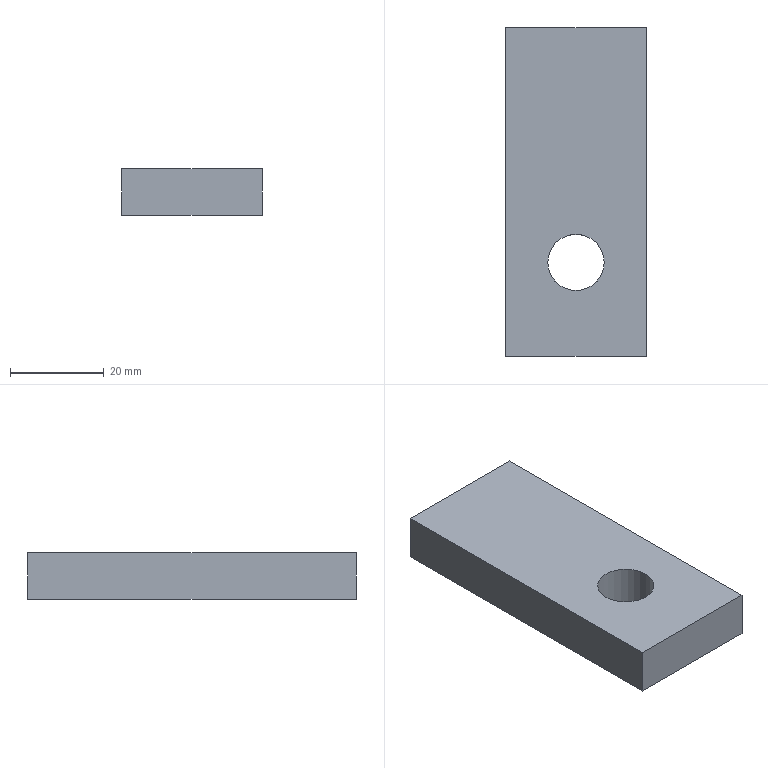Part | NX | features solid 2 | 1 solid | 7 faces | box 30 x 70 x 10 mm | volume 19869 mm3 | plane 6 | cylinder 1 | commonest cylinder face diameters 12 x1
STEP:
#1=CARTESIAN_POINT('',(664.,10.,-75.));
#2=VERTEX_POINT('',#1);
#3=CARTESIAN_POINT('',(670.,10.,-75.));
#4=DIRECTION('',(0.,0.,-1.));
#5=DIRECTION('',(-1.,0.,0.));
#6=AXIS2_PLACEMENT_3D('',#3,#4,#5);
#7=CIRCLE('',#6,6.);
#8=EDGE_CURVE('',#2,#2,#7,.F.);
#9=ORIENTED_EDGE('',*,*,#8,.F.);
#10=EDGE_LOOP('',(#9));
#11=FACE_BOUND('',#10,.T.);
#12=CARTESIAN_POINT('',(664.,10.,-65.));
#13=VERTEX_POINT('',#12);
#14=CARTESIAN_POINT('',(670.,10.,-65.));
#15=DIRECTION('',(0.,0.,-1.));
#16=DIRECTION('',(-1.,0.,0.));
#17=AXIS2_PLACEMENT_3D('',#14,#15,#16);
#18=CIRCLE('',#17,6.);
#19=EDGE_CURVE('',#13,#13,#18,.F.);
#20=ORIENTED_EDGE('',*,*,#19,.T.);
#21=EDGE_LOOP('',(#20));
#22=FACE_BOUND('',#21,.T.);
#23=CARTESIAN_POINT('',(670.,10.,-10.));
#24=DIRECTION('',(0.,0.,-1.));
#25=DIRECTION('',(-1.,0.,0.));
#26=AXIS2_PLACEMENT_3D('',#23,#24,#25);
#27=CYLINDRICAL_SURFACE('',#26,6.);
#28=ADVANCED_FACE('',(#11,#22),#27,.F.);
#29=CARTESIAN_POINT('',(685.,-10.,-65.));
#30=VERTEX_POINT('',#29);
#31=CARTESIAN_POINT('',(685.,-10.,-75.));
#32=VERTEX_POINT('',#31);
#33=CARTESIAN_POINT('',(685.,-10.,-10.));
#34=DIRECTION('',(0.,0.,1.));
#35=VECTOR('',#34,1000.);
#36=LINE('',#33,#35);
#37=EDGE_CURVE('',#30,#32,#36,.F.);
#38=ORIENTED_EDGE('',*,*,#37,.F.);
#39=CARTESIAN_POINT('',(655.,-10.,-65.));
#40=VERTEX_POINT('',#39);
#41=CARTESIAN_POINT('',(585.,-10.,-65.));
#42=DIRECTION('',(1.,0.,0.));
#43=VECTOR('',#42,1000.);
#44=LINE('',#41,#43);
#45=EDGE_CURVE('',#40,#30,#44,.T.);
#46=ORIENTED_EDGE('',*,*,#45,.F.);
#47=CARTESIAN_POINT('',(655.,-10.,-75.));
#48=VERTEX_POINT('',#47);
#49=CARTESIAN_POINT('',(655.,-10.,-10.));
#50=DIRECTION('',(0.,0.,1.));
#51=VECTOR('',#50,1000.);
#52=LINE('',#49,#51);
#53=EDGE_CURVE('',#40,#48,#52,.F.);
#54=ORIENTED_EDGE('',*,*,#53,.T.);
#55=CARTESIAN_POINT('',(585.,-10.,-75.));
#56=DIRECTION('',(1.,0.,0.));
#57=VECTOR('',#56,1000.);
#58=LINE('',#55,#57);
#59=EDGE_CURVE('',#32,#48,#58,.F.);
#60=ORIENTED_EDGE('',*,*,#59,.F.);
#61=EDGE_LOOP('',(#38,#46,#54,#60));
#62=FACE_BOUND('',#61,.T.);
#63=CARTESIAN_POINT('',(685.,-10.,-10.));
#64=DIRECTION('',(0.,1.,0.));
#65=DIRECTION('',(0.,0.,1.));
#66=AXIS2_PLACEMENT_3D('',#63,#64,#65);
#67=PLANE('',#66);
#68=ADVANCED_FACE('',(#62),#67,.F.);
#69=ORIENTED_EDGE('',*,*,#53,.F.);
#70=CARTESIAN_POINT('',(655.,60.,-65.));
#71=VERTEX_POINT('',#70);
#72=CARTESIAN_POINT('',(655.,90.,-65.));
#73=DIRECTION('',(0.,1.,0.));
#74=VECTOR('',#73,1000.);
#75=LINE('',#72,#74);
#76=EDGE_CURVE('',#71,#40,#75,.F.);
#77=ORIENTED_EDGE('',*,*,#76,.F.);
#78=CARTESIAN_POINT('',(655.,60.,-75.));
#79=VERTEX_POINT('',#78);
#80=CARTESIAN_POINT('',(655.,60.,-10.));
#81=DIRECTION('',(0.,0.,1.));
#82=VECTOR('',#81,1000.);
#83=LINE('',#80,#82);
#84=EDGE_CURVE('',#71,#79,#83,.F.);
#85=ORIENTED_EDGE('',*,*,#84,.T.);
#86=CARTESIAN_POINT('',(655.,205.,-75.));
#87=DIRECTION('',(0.,1.,0.));
#88=VECTOR('',#87,1000.);
#89=LINE('',#86,#88);
#90=EDGE_CURVE('',#79,#48,#89,.F.);
#91=ORIENTED_EDGE('',*,*,#90,.T.);
#92=EDGE_LOOP('',(#69,#77,#85,#91));
#93=FACE_BOUND('',#92,.T.);
#94=CARTESIAN_POINT('',(655.,205.,-10.));
#95=DIRECTION('',(1.,0.,0.));
#96=DIRECTION('',(0.,0.,-1.));
#97=AXIS2_PLACEMENT_3D('',#94,#95,#96);
#98=PLANE('',#97);
#99=ADVANCED_FACE('',(#93),#98,.F.);
#100=CARTESIAN_POINT('',(685.,60.,-75.));
#101=VERTEX_POINT('',#100);
#102=CARTESIAN_POINT('',(685.,205.,-75.));
#103=DIRECTION('',(0.,1.,0.));
#104=VECTOR('',#103,1000.);
#105=LINE('',#102,#104);
#106=EDGE_CURVE('',#101,#32,#105,.F.);
#107=ORIENTED_EDGE('',*,*,#106,.F.);
#108=CARTESIAN_POINT('',(685.,60.,-65.));
#109=VERTEX_POINT('',#108);
#110=CARTESIAN_POINT('',(685.,60.,-10.));
#111=DIRECTION('',(0.,0.,-1.));
#112=VECTOR('',#111,1000.);
#113=LINE('',#110,#112);
#114=EDGE_CURVE('',#101,#109,#113,.F.);
#115=ORIENTED_EDGE('',*,*,#114,.T.);
#116=CARTESIAN_POINT('',(685.,90.,-65.));
#117=DIRECTION('',(0.,1.,0.));
#118=VECTOR('',#117,1000.);
#119=LINE('',#116,#118);
#120=EDGE_CURVE('',#109,#30,#119,.F.);
#121=ORIENTED_EDGE('',*,*,#120,.T.);
#122=ORIENTED_EDGE('',*,*,#37,.T.);
#123=EDGE_LOOP('',(#107,#115,#121,#122));
#124=FACE_BOUND('',#123,.T.);
#125=CARTESIAN_POINT('',(685.,205.,-10.));
#126=DIRECTION('',(1.,0.,0.));
#127=DIRECTION('',(0.,0.,-1.));
#128=AXIS2_PLACEMENT_3D('',#125,#126,#127);
#129=PLANE('',#128);
#130=ADVANCED_FACE('',(#124),#129,.T.);
#131=ORIENTED_EDGE('',*,*,#120,.F.);
#132=CARTESIAN_POINT('',(585.,60.,-65.));
#133=DIRECTION('',(-1.,0.,0.));
#134=VECTOR('',#133,1000.);
#135=LINE('',#132,#134);
#136=EDGE_CURVE('',#109,#71,#135,.T.);
#137=ORIENTED_EDGE('',*,*,#136,.T.);
#138=ORIENTED_EDGE('',*,*,#76,.T.);
#139=ORIENTED_EDGE('',*,*,#45,.T.);
#140=EDGE_LOOP('',(#131,#137,#138,#139));
#141=FACE_BOUND('',#140,.T.);
#142=ORIENTED_EDGE('',*,*,#19,.F.);
#143=EDGE_LOOP('',(#142));
#144=FACE_BOUND('',#143,.T.);
#145=CARTESIAN_POINT('',(585.,225.,-65.));
#146=DIRECTION('',(0.,0.,-1.));
#147=DIRECTION('',(0.,1.,0.));
#148=AXIS2_PLACEMENT_3D('',#145,#146,#147);
#149=PLANE('',#148);
#150=ADVANCED_FACE('',(#141,#144),#149,.F.);
#151=ORIENTED_EDGE('',*,*,#90,.F.);
#152=CARTESIAN_POINT('',(585.,60.,-75.));
#153=DIRECTION('',(-1.,0.,0.));
#154=VECTOR('',#153,1000.);
#155=LINE('',#152,#154);
#156=EDGE_CURVE('',#79,#101,#155,.F.);
#157=ORIENTED_EDGE('',*,*,#156,.T.);
#158=ORIENTED_EDGE('',*,*,#106,.T.);
#159=ORIENTED_EDGE('',*,*,#59,.T.);
#160=EDGE_LOOP('',(#151,#157,#158,#159));
#161=FACE_BOUND('',#160,.T.);
#162=ORIENTED_EDGE('',*,*,#8,.T.);
#163=EDGE_LOOP('',(#162));
#164=FACE_BOUND('',#163,.T.);
#165=CARTESIAN_POINT('',(585.,225.,-75.));
#166=DIRECTION('',(0.,0.,-1.));
#167=DIRECTION('',(0.,1.,0.));
#168=AXIS2_PLACEMENT_3D('',#165,#166,#167);
#169=PLANE('',#168);
#170=ADVANCED_FACE('',(#161,#164),#169,.T.);
#171=ORIENTED_EDGE('',*,*,#136,.F.);
#172=ORIENTED_EDGE('',*,*,#114,.F.);
#173=ORIENTED_EDGE('',*,*,#156,.F.);
#174=ORIENTED_EDGE('',*,*,#84,.F.);
#175=EDGE_LOOP('',(#171,#172,#173,#174));
#176=FACE_BOUND('',#175,.T.);
#177=CARTESIAN_POINT('',(670.,60.,-10.));
#178=DIRECTION('',(0.,-1.,0.));
#179=DIRECTION('',(0.,0.,-1.));
#180=AXIS2_PLACEMENT_3D('',#177,#178,#179);
#181=PLANE('',#180);
#182=ADVANCED_FACE('',(#176),#181,.F.);
#183=CLOSED_SHELL('',(#28,#68,#99,#130,#150,#170,#182));
#184=MANIFOLD_SOLID_BREP('',#183);
#185=(LENGTH_UNIT()NAMED_UNIT(*)SI_UNIT(.MILLI.,.METRE.));
#186=UNCERTAINTY_MEASURE_WITH_UNIT(LENGTH_MEASURE(0.00001),#185,'','');
#187=(NAMED_UNIT(*)PLANE_ANGLE_UNIT()SI_UNIT($,.RADIAN.));
#188=(NAMED_UNIT(*)SI_UNIT($,.STERADIAN.)SOLID_ANGLE_UNIT());
#189=(GEOMETRIC_REPRESENTATION_CONTEXT(3)GLOBAL_UNCERTAINTY_ASSIGNED_CONTEXT((#186))GLOBAL_UNIT_ASSIGNED_CONTEXT((#185,#187,#188))REPRESENTATION_CONTEXT('',''));
#190=ADVANCED_BREP_SHAPE_REPRESENTATION('',(#184),#189);